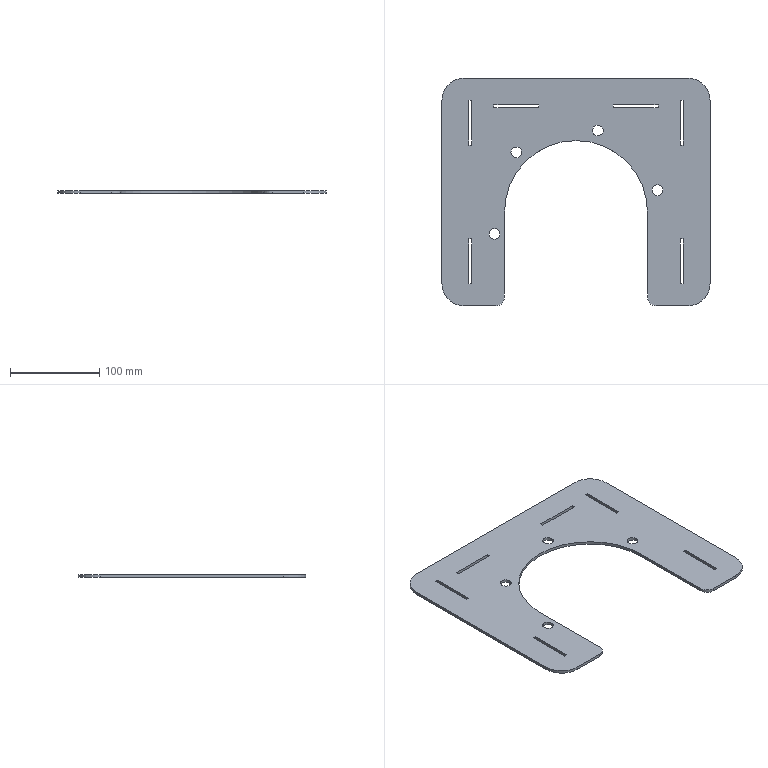Part | SolidWorks | features FlatPattern 1, SMBaseFlange 1, SheetMetal 1 | 1 solid | 48 faces | box 300 x 255 x 3.2 mm | volume 152496 mm3 | plane 33 | cylinder 15 | commonest cylinder face diameters 12 x8 50 x4 20 x2 160 x1